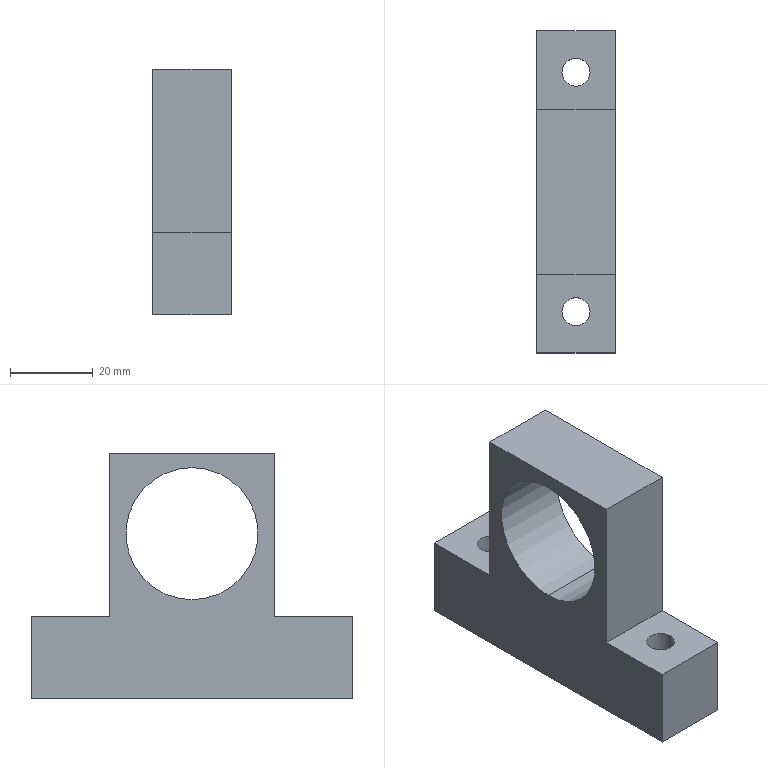Part | STEP file | PN_0052 secondary end seat | 1 solid | 16 faces | box 19 x 78 x 59.5 mm | volume 42927 mm3 | plane 10 | cylinder 6 | commonest cylinder face diameters 6.8 x4 32 x2
STEP:
#1=CARTESIAN_POINT('',(0.,0.,0.));
#2=DIRECTION('',(0.,0.,1.));
#3=DIRECTION('',(1.,0.,0.));
#4=AXIS2_PLACEMENT_3D('',#1,#2,#3);
#5=CARTESIAN_POINT('',(3.4,29.,0.));
#6=VERTEX_POINT('',#5);
#7=CARTESIAN_POINT('',(3.4,29.,20.));
#8=VERTEX_POINT('',#7);
#9=CARTESIAN_POINT('',(3.4,29.,20.));
#10=DIRECTION('',(0.,0.,1.));
#11=VECTOR('',#10,1.);
#12=LINE('',#9,#11);
#13=CARTESIAN_POINT('',(0.,29.,20.));
#14=DIRECTION('',(0.,0.,1.));
#15=DIRECTION('',(1.,0.,0.));
#16=AXIS2_PLACEMENT_3D('',#13,#14,#15);
#17=CYLINDRICAL_SURFACE('',#16,3.4);
#18=CARTESIAN_POINT('',(6.283,0.));
#19=DIRECTION('',(0.,1.));
#20=VECTOR('',#19,1.);
#21=LINE('',#18,#20);
#22=(GEOMETRIC_REPRESENTATION_CONTEXT(2)PARAMETRIC_REPRESENTATION_CONTEXT()REPRESENTATION_CONTEXT('',''));
#23=DEFINITIONAL_REPRESENTATION('',(#21),#22);
#24=PCURVE('',#17,#23);
#25=CARTESIAN_POINT('',(0.,29.,20.));
#26=DIRECTION('',(0.,0.,1.));
#27=DIRECTION('',(1.,0.,0.));
#28=AXIS2_PLACEMENT_3D('',#25,#26,#27);
#29=CYLINDRICAL_SURFACE('',#28,3.4);
#30=CARTESIAN_POINT('',(0.,0.));
#31=DIRECTION('',(0.,1.));
#32=VECTOR('',#31,1.);
#33=LINE('',#30,#32);
#34=(GEOMETRIC_REPRESENTATION_CONTEXT(2)PARAMETRIC_REPRESENTATION_CONTEXT()REPRESENTATION_CONTEXT('',''));
#35=DEFINITIONAL_REPRESENTATION('',(#33),#34);
#36=PCURVE('',#29,#35);
#37=SURFACE_CURVE('',#12,(#24,#36),.PCURVE_S1.);
#38=EDGE_CURVE('',#6,#8,#37,.T.);
#39=ORIENTED_EDGE('',*,*,#38,.T.);
#40=CARTESIAN_POINT('',(-3.4,29.,20.));
#41=VERTEX_POINT('',#40);
#42=CARTESIAN_POINT('',(0.,29.,20.));
#43=DIRECTION('',(0.,0.,1.));
#44=DIRECTION('',(1.,0.,0.));
#45=AXIS2_PLACEMENT_3D('',#42,#43,#44);
#46=CIRCLE('',#45,3.4);
#47=CARTESIAN_POINT('',(0.,0.));
#48=DIRECTION('',(1.,0.));
#49=VECTOR('',#48,1.);
#50=LINE('',#47,#49);
#51=(GEOMETRIC_REPRESENTATION_CONTEXT(2)PARAMETRIC_REPRESENTATION_CONTEXT()REPRESENTATION_CONTEXT('',''));
#52=DEFINITIONAL_REPRESENTATION('',(#50),#51);
#53=PCURVE('',#17,#52);
#54=CARTESIAN_POINT('',(9.5,39.,20.));
#55=DIRECTION('',(0.,0.,-1.));
#56=DIRECTION('',(0.,1.,0.));
#57=AXIS2_PLACEMENT_3D('',#54,#55,#56);
#58=PLANE('',#57);
#59=CARTESIAN_POINT('',(-10.,-6.1));
#60=CARTESIAN_POINT('',(-4.111,-6.1));
#61=CARTESIAN_POINT('',(-7.056,-11.2));
#62=CARTESIAN_POINT('',(-10.,-16.3));
#63=CARTESIAN_POINT('',(-12.944,-11.2));
#64=CARTESIAN_POINT('',(-15.889,-6.1));
#65=CARTESIAN_POINT('',(-10.,-6.1));
#66=(BOUNDED_CURVE()B_SPLINE_CURVE(2,(#59,#60,#61,#62,#63,#64,#65),.UNSPECIFIED.,.T.,.F.)B_SPLINE_CURVE_WITH_KNOTS((1,2,2,2,2,1),(-2.094,0.,2.094,4.189,6.283,8.378),.UNSPECIFIED.)CURVE()GEOMETRIC_REPRESENTATION_ITEM()RATIONAL_B_SPLINE_CURVE((1.,0.5,1.,0.5,1.,0.5,1.))REPRESENTATION_ITEM(''));
#67=(GEOMETRIC_REPRESENTATION_CONTEXT(2)PARAMETRIC_REPRESENTATION_CONTEXT()REPRESENTATION_CONTEXT('',''));
#68=DEFINITIONAL_REPRESENTATION('',(#66),#67);
#69=PCURVE('',#58,#68);
#70=SURFACE_CURVE('',#46,(#53,#69),.PCURVE_S1.);
#71=EDGE_CURVE('',#41,#8,#70,.T.);
#72=ORIENTED_EDGE('',*,*,#71,.F.);
#73=CARTESIAN_POINT('',(-3.4,29.,0.));
#74=VERTEX_POINT('',#73);
#75=CARTESIAN_POINT('',(-3.4,29.,20.));
#76=DIRECTION('',(0.,0.,1.));
#77=VECTOR('',#76,1.);
#78=LINE('',#75,#77);
#79=CARTESIAN_POINT('',(3.142,0.));
#80=DIRECTION('',(0.,1.));
#81=VECTOR('',#80,1.);
#82=LINE('',#79,#81);
#83=(GEOMETRIC_REPRESENTATION_CONTEXT(2)PARAMETRIC_REPRESENTATION_CONTEXT()REPRESENTATION_CONTEXT('',''));
#84=DEFINITIONAL_REPRESENTATION('',(#82),#83);
#85=PCURVE('',#17,#84);
#86=CARTESIAN_POINT('',(3.142,0.));
#87=DIRECTION('',(0.,1.));
#88=VECTOR('',#87,1.);
#89=LINE('',#86,#88);
#90=(GEOMETRIC_REPRESENTATION_CONTEXT(2)PARAMETRIC_REPRESENTATION_CONTEXT()REPRESENTATION_CONTEXT('',''));
#91=DEFINITIONAL_REPRESENTATION('',(#89),#90);
#92=PCURVE('',#29,#91);
#93=SURFACE_CURVE('',#78,(#85,#92),.PCURVE_S1.);
#94=EDGE_CURVE('',#74,#41,#93,.T.);
#95=ORIENTED_EDGE('',*,*,#94,.F.);
#96=CARTESIAN_POINT('',(0.,29.,0.));
#97=DIRECTION('',(0.,0.,1.));
#98=DIRECTION('',(1.,0.,0.));
#99=AXIS2_PLACEMENT_3D('',#96,#97,#98);
#100=CIRCLE('',#99,3.4);
#101=CARTESIAN_POINT('',(0.,-20.));
#102=DIRECTION('',(1.,0.));
#103=VECTOR('',#102,1.);
#104=LINE('',#101,#103);
#105=(GEOMETRIC_REPRESENTATION_CONTEXT(2)PARAMETRIC_REPRESENTATION_CONTEXT()REPRESENTATION_CONTEXT('',''));
#106=DEFINITIONAL_REPRESENTATION('',(#104),#105);
#107=PCURVE('',#17,#106);
#108=CARTESIAN_POINT('',(9.5,-39.,0.));
#109=DIRECTION('',(0.,0.,1.));
#110=DIRECTION('',(0.,-1.,0.));
#111=AXIS2_PLACEMENT_3D('',#108,#109,#110);
#112=PLANE('',#111);
#113=CARTESIAN_POINT('',(-68.,-9.5));
#114=DIRECTION('',(0.,1.));
#115=AXIS2_PLACEMENT_2D('',#113,#114);
#116=CIRCLE('',#115,3.4);
#117=(GEOMETRIC_REPRESENTATION_CONTEXT(2)PARAMETRIC_REPRESENTATION_CONTEXT()REPRESENTATION_CONTEXT('',''));
#118=DEFINITIONAL_REPRESENTATION('',(#116),#117);
#119=PCURVE('',#112,#118);
#120=SURFACE_CURVE('',#100,(#107,#119),.PCURVE_S1.);
#121=EDGE_CURVE('',#74,#6,#120,.T.);
#122=ORIENTED_EDGE('',*,*,#121,.T.);
#123=EDGE_LOOP('',(#39,#72,#95,#122));
#124=FACE_BOUND('',#123,.F.);
#125=ADVANCED_FACE('',(#124),#17,.F.);
#126=CARTESIAN_POINT('',(3.4,-29.,0.));
#127=VERTEX_POINT('',#126);
#128=CARTESIAN_POINT('',(3.4,-29.,20.));
#129=VERTEX_POINT('',#128);
#130=CARTESIAN_POINT('',(3.4,-29.,20.));
#131=DIRECTION('',(0.,0.,1.));
#132=VECTOR('',#131,1.);
#133=LINE('',#130,#132);
#134=CARTESIAN_POINT('',(0.,-29.,20.));
#135=DIRECTION('',(0.,0.,1.));
#136=DIRECTION('',(1.,0.,0.));
#137=AXIS2_PLACEMENT_3D('',#134,#135,#136);
#138=CYLINDRICAL_SURFACE('',#137,3.4);
#139=CARTESIAN_POINT('',(6.283,0.));
#140=DIRECTION('',(0.,1.));
#141=VECTOR('',#140,1.);
#142=LINE('',#139,#141);
#143=(GEOMETRIC_REPRESENTATION_CONTEXT(2)PARAMETRIC_REPRESENTATION_CONTEXT()REPRESENTATION_CONTEXT('',''));
#144=DEFINITIONAL_REPRESENTATION('',(#142),#143);
#145=PCURVE('',#138,#144);
#146=CARTESIAN_POINT('',(0.,-29.,20.));
#147=DIRECTION('',(0.,0.,1.));
#148=DIRECTION('',(1.,0.,0.));
#149=AXIS2_PLACEMENT_3D('',#146,#147,#148);
#150=CYLINDRICAL_SURFACE('',#149,3.4);
#151=CARTESIAN_POINT('',(0.,0.));
#152=DIRECTION('',(0.,1.));
#153=VECTOR('',#152,1.);
#154=LINE('',#151,#153);
#155=(GEOMETRIC_REPRESENTATION_CONTEXT(2)PARAMETRIC_REPRESENTATION_CONTEXT()REPRESENTATION_CONTEXT('',''));
#156=DEFINITIONAL_REPRESENTATION('',(#154),#155);
#157=PCURVE('',#150,#156);
#158=SURFACE_CURVE('',#133,(#145,#157),.PCURVE_S1.);
#159=EDGE_CURVE('',#127,#129,#158,.T.);
#160=ORIENTED_EDGE('',*,*,#159,.T.);
#161=CARTESIAN_POINT('',(-3.4,-29.,20.));
#162=VERTEX_POINT('',#161);
#163=CARTESIAN_POINT('',(0.,-29.,20.));
#164=DIRECTION('',(0.,0.,1.));
#165=DIRECTION('',(1.,0.,0.));
#166=AXIS2_PLACEMENT_3D('',#163,#164,#165);
#167=CIRCLE('',#166,3.4);
#168=CARTESIAN_POINT('',(0.,0.));
#169=DIRECTION('',(1.,0.));
#170=VECTOR('',#169,1.);
#171=LINE('',#168,#170);
#172=(GEOMETRIC_REPRESENTATION_CONTEXT(2)PARAMETRIC_REPRESENTATION_CONTEXT()REPRESENTATION_CONTEXT('',''));
#173=DEFINITIONAL_REPRESENTATION('',(#171),#172);
#174=PCURVE('',#138,#173);
#175=CARTESIAN_POINT('',(9.5,-20.,20.));
#176=DIRECTION('',(0.,0.,-1.));
#177=DIRECTION('',(0.,1.,0.));
#178=AXIS2_PLACEMENT_3D('',#175,#176,#177);
#179=PLANE('',#178);
#180=CARTESIAN_POINT('',(-9.,-6.1));
#181=CARTESIAN_POINT('',(-3.111,-6.1));
#182=CARTESIAN_POINT('',(-6.056,-11.2));
#183=CARTESIAN_POINT('',(-9.,-16.3));
#184=CARTESIAN_POINT('',(-11.944,-11.2));
#185=CARTESIAN_POINT('',(-14.889,-6.1));
#186=CARTESIAN_POINT('',(-9.,-6.1));
#187=(BOUNDED_CURVE()B_SPLINE_CURVE(2,(#180,#181,#182,#183,#184,#185,#186),.UNSPECIFIED.,.T.,.F.)B_SPLINE_CURVE_WITH_KNOTS((1,2,2,2,2,1),(-2.094,0.,2.094,4.189,6.283,8.378),.UNSPECIFIED.)CURVE()GEOMETRIC_REPRESENTATION_ITEM()RATIONAL_B_SPLINE_CURVE((1.,0.5,1.,0.5,1.,0.5,1.))REPRESENTATION_ITEM(''));
#188=(GEOMETRIC_REPRESENTATION_CONTEXT(2)PARAMETRIC_REPRESENTATION_CONTEXT()REPRESENTATION_CONTEXT('',''));
#189=DEFINITIONAL_REPRESENTATION('',(#187),#188);
#190=PCURVE('',#179,#189);
#191=SURFACE_CURVE('',#167,(#174,#190),.PCURVE_S1.);
#192=EDGE_CURVE('',#162,#129,#191,.T.);
#193=ORIENTED_EDGE('',*,*,#192,.F.);
#194=CARTESIAN_POINT('',(-3.4,-29.,0.));
#195=VERTEX_POINT('',#194);
#196=CARTESIAN_POINT('',(-3.4,-29.,20.));
#197=DIRECTION('',(0.,0.,1.));
#198=VECTOR('',#197,1.);
#199=LINE('',#196,#198);
#200=CARTESIAN_POINT('',(3.142,0.));
#201=DIRECTION('',(0.,1.));
#202=VECTOR('',#201,1.);
#203=LINE('',#200,#202);
#204=(GEOMETRIC_REPRESENTATION_CONTEXT(2)PARAMETRIC_REPRESENTATION_CONTEXT()REPRESENTATION_CONTEXT('',''));
#205=DEFINITIONAL_REPRESENTATION('',(#203),#204);
#206=PCURVE('',#138,#205);
#207=CARTESIAN_POINT('',(3.142,0.));
#208=DIRECTION('',(0.,1.));
#209=VECTOR('',#208,1.);
#210=LINE('',#207,#209);
#211=(GEOMETRIC_REPRESENTATION_CONTEXT(2)PARAMETRIC_REPRESENTATION_CONTEXT()REPRESENTATION_CONTEXT('',''));
#212=DEFINITIONAL_REPRESENTATION('',(#210),#211);
#213=PCURVE('',#150,#212);
#214=SURFACE_CURVE('',#199,(#206,#213),.PCURVE_S1.);
#215=EDGE_CURVE('',#195,#162,#214,.T.);
#216=ORIENTED_EDGE('',*,*,#215,.F.);
#217=CARTESIAN_POINT('',(0.,-29.,0.));
#218=DIRECTION('',(0.,0.,1.));
#219=DIRECTION('',(1.,0.,0.));
#220=AXIS2_PLACEMENT_3D('',#217,#218,#219);
#221=CIRCLE('',#220,3.4);
#222=CARTESIAN_POINT('',(0.,-20.));
#223=DIRECTION('',(1.,0.));
#224=VECTOR('',#223,1.);
#225=LINE('',#222,#224);
#226=(GEOMETRIC_REPRESENTATION_CONTEXT(2)PARAMETRIC_REPRESENTATION_CONTEXT()REPRESENTATION_CONTEXT('',''));
#227=DEFINITIONAL_REPRESENTATION('',(#225),#226);
#228=PCURVE('',#138,#227);
#229=CARTESIAN_POINT('',(-10.,-9.5));
#230=DIRECTION('',(0.,1.));
#231=AXIS2_PLACEMENT_2D('',#229,#230);
#232=CIRCLE('',#231,3.4);
#233=(GEOMETRIC_REPRESENTATION_CONTEXT(2)PARAMETRIC_REPRESENTATION_CONTEXT()REPRESENTATION_CONTEXT('',''));
#234=DEFINITIONAL_REPRESENTATION('',(#232),#233);
#235=PCURVE('',#112,#234);
#236=SURFACE_CURVE('',#221,(#228,#235),.PCURVE_S1.);
#237=EDGE_CURVE('',#195,#127,#236,.T.);
#238=ORIENTED_EDGE('',*,*,#237,.T.);
#239=EDGE_LOOP('',(#160,#193,#216,#238));
#240=FACE_BOUND('',#239,.F.);
#241=ADVANCED_FACE('',(#240),#138,.F.);
#242=CARTESIAN_POINT('',(-9.5,0.,24.));
#243=VERTEX_POINT('',#242);
#244=CARTESIAN_POINT('',(9.5,0.,24.));
#245=VERTEX_POINT('',#244);
#246=CARTESIAN_POINT('',(-9.5,0.,24.));
#247=DIRECTION('',(1.,0.,0.));
#248=VECTOR('',#247,1.);
#249=LINE('',#246,#248);
#250=CARTESIAN_POINT('',(-9.5,0.,40.));
#251=DIRECTION('',(1.,0.,0.));
#252=DIRECTION('',(0.,0.,-1.));
#253=AXIS2_PLACEMENT_3D('',#250,#251,#252);
#254=CYLINDRICAL_SURFACE('',#253,16.);
#255=CARTESIAN_POINT('',(6.283,0.));
#256=DIRECTION('',(0.,1.));
#257=VECTOR('',#256,1.);
#258=LINE('',#255,#257);
#259=(GEOMETRIC_REPRESENTATION_CONTEXT(2)PARAMETRIC_REPRESENTATION_CONTEXT()REPRESENTATION_CONTEXT('',''));
#260=DEFINITIONAL_REPRESENTATION('',(#258),#259);
#261=PCURVE('',#254,#260);
#262=CARTESIAN_POINT('',(-9.5,0.,40.));
#263=DIRECTION('',(1.,0.,0.));
#264=DIRECTION('',(0.,0.,-1.));
#265=AXIS2_PLACEMENT_3D('',#262,#263,#264);
#266=CYLINDRICAL_SURFACE('',#265,16.);
#267=CARTESIAN_POINT('',(0.,0.));
#268=DIRECTION('',(0.,1.));
#269=VECTOR('',#268,1.);
#270=LINE('',#267,#269);
#271=(GEOMETRIC_REPRESENTATION_CONTEXT(2)PARAMETRIC_REPRESENTATION_CONTEXT()REPRESENTATION_CONTEXT('',''));
#272=DEFINITIONAL_REPRESENTATION('',(#270),#271);
#273=PCURVE('',#266,#272);
#274=SURFACE_CURVE('',#249,(#261,#273),.PCURVE_S1.);
#275=EDGE_CURVE('',#243,#245,#274,.T.);
#276=ORIENTED_EDGE('',*,*,#275,.T.);
#277=CARTESIAN_POINT('',(9.5,0.,56.));
#278=VERTEX_POINT('',#277);
#279=CARTESIAN_POINT('',(9.5,0.,40.));
#280=DIRECTION('',(1.,0.,0.));
#281=DIRECTION('',(0.,0.,-1.));
#282=AXIS2_PLACEMENT_3D('',#279,#280,#281);
#283=CIRCLE('',#282,16.);
#284=CARTESIAN_POINT('',(0.,19.));
#285=DIRECTION('',(1.,0.));
#286=VECTOR('',#285,1.);
#287=LINE('',#284,#286);
#288=(GEOMETRIC_REPRESENTATION_CONTEXT(2)PARAMETRIC_REPRESENTATION_CONTEXT()REPRESENTATION_CONTEXT('',''));
#289=DEFINITIONAL_REPRESENTATION('',(#287),#288);
#290=PCURVE('',#254,#289);
#291=CARTESIAN_POINT('',(9.5,0.,0.));
#292=DIRECTION('',(1.,0.,0.));
#293=DIRECTION('',(0.,0.,-1.));
#294=AXIS2_PLACEMENT_3D('',#291,#292,#293);
#295=PLANE('',#294);
#296=CARTESIAN_POINT('',(-40.,0.));
#297=DIRECTION('',(1.,0.));
#298=AXIS2_PLACEMENT_2D('',#296,#297);
#299=CIRCLE('',#298,16.);
#300=(GEOMETRIC_REPRESENTATION_CONTEXT(2)PARAMETRIC_REPRESENTATION_CONTEXT()REPRESENTATION_CONTEXT('',''));
#301=DEFINITIONAL_REPRESENTATION('',(#299),#300);
#302=PCURVE('',#295,#301);
#303=SURFACE_CURVE('',#283,(#290,#302),.PCURVE_S1.);
#304=EDGE_CURVE('',#278,#245,#303,.T.);
#305=ORIENTED_EDGE('',*,*,#304,.F.);
#306=CARTESIAN_POINT('',(-9.5,0.,56.));
#307=VERTEX_POINT('',#306);
#308=CARTESIAN_POINT('',(-9.5,0.,56.));
#309=DIRECTION('',(1.,0.,0.));
#310=VECTOR('',#309,1.);
#311=LINE('',#308,#310);
#312=CARTESIAN_POINT('',(3.142,0.));
#313=DIRECTION('',(0.,1.));
#314=VECTOR('',#313,1.);
#315=LINE('',#312,#314);
#316=(GEOMETRIC_REPRESENTATION_CONTEXT(2)PARAMETRIC_REPRESENTATION_CONTEXT()REPRESENTATION_CONTEXT('',''));
#317=DEFINITIONAL_REPRESENTATION('',(#315),#316);
#318=PCURVE('',#254,#317);
#319=CARTESIAN_POINT('',(3.142,0.));
#320=DIRECTION('',(0.,1.));
#321=VECTOR('',#320,1.);
#322=LINE('',#319,#321);
#323=(GEOMETRIC_REPRESENTATION_CONTEXT(2)PARAMETRIC_REPRESENTATION_CONTEXT()REPRESENTATION_CONTEXT('',''));
#324=DEFINITIONAL_REPRESENTATION('',(#322),#323);
#325=PCURVE('',#266,#324);
#326=SURFACE_CURVE('',#311,(#318,#325),.PCURVE_S1.);
#327=EDGE_CURVE('',#307,#278,#326,.T.);
#328=ORIENTED_EDGE('',*,*,#327,.F.);
#329=CARTESIAN_POINT('',(-9.5,0.,40.));
#330=DIRECTION('',(1.,0.,0.));
#331=DIRECTION('',(0.,0.,-1.));
#332=AXIS2_PLACEMENT_3D('',#329,#330,#331);
#333=CIRCLE('',#332,16.);
#334=CARTESIAN_POINT('',(0.,0.));
#335=DIRECTION('',(1.,0.));
#336=VECTOR('',#335,1.);
#337=LINE('',#334,#336);
#338=(GEOMETRIC_REPRESENTATION_CONTEXT(2)PARAMETRIC_REPRESENTATION_CONTEXT()REPRESENTATION_CONTEXT('',''));
#339=DEFINITIONAL_REPRESENTATION('',(#337),#338);
#340=PCURVE('',#254,#339);
#341=CARTESIAN_POINT('',(-9.5,0.,0.));
#342=DIRECTION('',(1.,0.,0.));
#343=DIRECTION('',(0.,0.,-1.));
#344=AXIS2_PLACEMENT_3D('',#341,#342,#343);
#345=PLANE('',#344);
#346=CARTESIAN_POINT('',(-40.,0.));
#347=DIRECTION('',(1.,0.));
#348=AXIS2_PLACEMENT_2D('',#346,#347);
#349=CIRCLE('',#348,16.);
#350=(GEOMETRIC_REPRESENTATION_CONTEXT(2)PARAMETRIC_REPRESENTATION_CONTEXT()REPRESENTATION_CONTEXT('',''));
#351=DEFINITIONAL_REPRESENTATION('',(#349),#350);
#352=PCURVE('',#345,#351);
#353=SURFACE_CURVE('',#333,(#340,#352),.PCURVE_S1.);
#354=EDGE_CURVE('',#307,#243,#353,.T.);
#355=ORIENTED_EDGE('',*,*,#354,.T.);
#356=EDGE_LOOP('',(#276,#305,#328,#355));
#357=FACE_BOUND('',#356,.F.);
#358=ADVANCED_FACE('',(#357),#254,.F.);
#359=CARTESIAN_POINT('',(0.,29.,0.));
#360=DIRECTION('',(0.,0.,1.));
#361=DIRECTION('',(1.,0.,0.));
#362=AXIS2_PLACEMENT_3D('',#359,#360,#361);
#363=CIRCLE('',#362,3.4);
#364=CARTESIAN_POINT('',(-68.,-9.5));
#365=DIRECTION('',(0.,1.));
#366=AXIS2_PLACEMENT_2D('',#364,#365);
#367=CIRCLE('',#366,3.4);
#368=(GEOMETRIC_REPRESENTATION_CONTEXT(2)PARAMETRIC_REPRESENTATION_CONTEXT()REPRESENTATION_CONTEXT('',''));
#369=DEFINITIONAL_REPRESENTATION('',(#367),#368);
#370=PCURVE('',#112,#369);
#371=CARTESIAN_POINT('',(0.,-20.));
#372=DIRECTION('',(1.,0.));
#373=VECTOR('',#372,1.);
#374=LINE('',#371,#373);
#375=(GEOMETRIC_REPRESENTATION_CONTEXT(2)PARAMETRIC_REPRESENTATION_CONTEXT()REPRESENTATION_CONTEXT('',''));
#376=DEFINITIONAL_REPRESENTATION('',(#374),#375);
#377=PCURVE('',#29,#376);
#378=SURFACE_CURVE('',#363,(#370,#377),.PCURVE_S1.);
#379=EDGE_CURVE('',#6,#74,#378,.T.);
#380=ORIENTED_EDGE('',*,*,#379,.T.);
#381=ORIENTED_EDGE('',*,*,#121,.T.);
#382=EDGE_LOOP('',(#380,#381));
#383=FACE_BOUND('',#382,.T.);
#384=CARTESIAN_POINT('',(0.,-29.,0.));
#385=DIRECTION('',(0.,0.,1.));
#386=DIRECTION('',(1.,0.,0.));
#387=AXIS2_PLACEMENT_3D('',#384,#385,#386);
#388=CIRCLE('',#387,3.4);
#389=CARTESIAN_POINT('',(-10.,-9.5));
#390=DIRECTION('',(0.,1.));
#391=AXIS2_PLACEMENT_2D('',#389,#390);
#392=CIRCLE('',#391,3.4);
#393=(GEOMETRIC_REPRESENTATION_CONTEXT(2)PARAMETRIC_REPRESENTATION_CONTEXT()REPRESENTATION_CONTEXT('',''));
#394=DEFINITIONAL_REPRESENTATION('',(#392),#393);
#395=PCURVE('',#112,#394);
#396=CARTESIAN_POINT('',(0.,-20.));
#397=DIRECTION('',(1.,0.));
#398=VECTOR('',#397,1.);
#399=LINE('',#396,#398);
#400=(GEOMETRIC_REPRESENTATION_CONTEXT(2)PARAMETRIC_REPRESENTATION_CONTEXT()REPRESENTATION_CONTEXT('',''));
#401=DEFINITIONAL_REPRESENTATION('',(#399),#400);
#402=PCURVE('',#150,#401);
#403=SURFACE_CURVE('',#388,(#395,#402),.PCURVE_S1.);
#404=EDGE_CURVE('',#127,#195,#403,.T.);
#405=ORIENTED_EDGE('',*,*,#404,.T.);
#406=ORIENTED_EDGE('',*,*,#237,.T.);
#407=EDGE_LOOP('',(#405,#406));
#408=FACE_BOUND('',#407,.T.);
#409=CARTESIAN_POINT('',(-9.5,-39.,0.));
#410=VERTEX_POINT('',#409);
#411=CARTESIAN_POINT('',(-9.5,39.,0.));
#412=VERTEX_POINT('',#411);
#413=CARTESIAN_POINT('',(-9.5,-39.,0.));
#414=DIRECTION('',(0.,1.,0.));
#415=VECTOR('',#414,1.);
#416=LINE('',#413,#415);
#417=CARTESIAN_POINT('',(0.,-19.));
#418=DIRECTION('',(-1.,0.));
#419=VECTOR('',#418,1.);
#420=LINE('',#417,#419);
#421=(GEOMETRIC_REPRESENTATION_CONTEXT(2)PARAMETRIC_REPRESENTATION_CONTEXT()REPRESENTATION_CONTEXT('',''));
#422=DEFINITIONAL_REPRESENTATION('',(#420),#421);
#423=PCURVE('',#112,#422);
#424=CARTESIAN_POINT('',(0.,-39.));
#425=DIRECTION('',(0.,1.));
#426=VECTOR('',#425,1.);
#427=LINE('',#424,#426);
#428=(GEOMETRIC_REPRESENTATION_CONTEXT(2)PARAMETRIC_REPRESENTATION_CONTEXT()REPRESENTATION_CONTEXT('',''));
#429=DEFINITIONAL_REPRESENTATION('',(#427),#428);
#430=PCURVE('',#345,#429);
#431=SURFACE_CURVE('',#416,(#423,#430),.PCURVE_S1.);
#432=EDGE_CURVE('',#410,#412,#431,.T.);
#433=ORIENTED_EDGE('',*,*,#432,.T.);
#434=CARTESIAN_POINT('',(9.5,39.,0.));
#435=VERTEX_POINT('',#434);
#436=CARTESIAN_POINT('',(9.5,39.,0.));
#437=DIRECTION('',(-1.,0.,0.));
#438=VECTOR('',#437,1.);
#439=LINE('',#436,#438);
#440=CARTESIAN_POINT('',(-78.,0.));
#441=DIRECTION('',(0.,-1.));
#442=VECTOR('',#441,1.);
#443=LINE('',#440,#442);
#444=(GEOMETRIC_REPRESENTATION_CONTEXT(2)PARAMETRIC_REPRESENTATION_CONTEXT()REPRESENTATION_CONTEXT('',''));
#445=DEFINITIONAL_REPRESENTATION('',(#443),#444);
#446=PCURVE('',#112,#445);
#447=CARTESIAN_POINT('',(9.5,39.,0.));
#448=DIRECTION('',(0.,-1.,0.));
#449=DIRECTION('',(0.,0.,-1.));
#450=AXIS2_PLACEMENT_3D('',#447,#448,#449);
#451=PLANE('',#450);
#452=CARTESIAN_POINT('',(0.,0.));
#453=DIRECTION('',(0.,-1.));
#454=VECTOR('',#453,1.);
#455=LINE('',#452,#454);
#456=(GEOMETRIC_REPRESENTATION_CONTEXT(2)PARAMETRIC_REPRESENTATION_CONTEXT()REPRESENTATION_CONTEXT('',''));
#457=DEFINITIONAL_REPRESENTATION('',(#455),#456);
#458=PCURVE('',#451,#457);
#459=SURFACE_CURVE('',#439,(#446,#458),.PCURVE_S1.);
#460=EDGE_CURVE('',#435,#412,#459,.T.);
#461=ORIENTED_EDGE('',*,*,#460,.F.);
#462=CARTESIAN_POINT('',(9.5,-39.,0.));
#463=VERTEX_POINT('',#462);
#464=CARTESIAN_POINT('',(9.5,-39.,0.));
#465=DIRECTION('',(0.,1.,0.));
#466=VECTOR('',#465,1.);
#467=LINE('',#464,#466);
#468=CARTESIAN_POINT('',(0.,0.));
#469=DIRECTION('',(-1.,0.));
#470=VECTOR('',#469,1.);
#471=LINE('',#468,#470);
#472=(GEOMETRIC_REPRESENTATION_CONTEXT(2)PARAMETRIC_REPRESENTATION_CONTEXT()REPRESENTATION_CONTEXT('',''));
#473=DEFINITIONAL_REPRESENTATION('',(#471),#472);
#474=PCURVE('',#112,#473);
#475=CARTESIAN_POINT('',(0.,-39.));
#476=DIRECTION('',(0.,1.));
#477=VECTOR('',#476,1.);
#478=LINE('',#475,#477);
#479=(GEOMETRIC_REPRESENTATION_CONTEXT(2)PARAMETRIC_REPRESENTATION_CONTEXT()REPRESENTATION_CONTEXT('',''));
#480=DEFINITIONAL_REPRESENTATION('',(#478),#479);
#481=PCURVE('',#295,#480);
#482=SURFACE_CURVE('',#467,(#474,#481),.PCURVE_S1.);
#483=EDGE_CURVE('',#463,#435,#482,.T.);
#484=ORIENTED_EDGE('',*,*,#483,.F.);
#485=CARTESIAN_POINT('',(9.5,-39.,0.));
#486=DIRECTION('',(-1.,0.,0.));
#487=VECTOR('',#486,1.);
#488=LINE('',#485,#487);
#489=CARTESIAN_POINT('',(0.,0.));
#490=DIRECTION('',(0.,-1.));
#491=VECTOR('',#490,1.);
#492=LINE('',#489,#491);
#493=(GEOMETRIC_REPRESENTATION_CONTEXT(2)PARAMETRIC_REPRESENTATION_CONTEXT()REPRESENTATION_CONTEXT('',''));
#494=DEFINITIONAL_REPRESENTATION('',(#492),#493);
#495=PCURVE('',#112,#494);
#496=CARTESIAN_POINT('',(9.5,-39.,0.));
#497=DIRECTION('',(0.,1.,0.));
#498=DIRECTION('',(0.,0.,1.));
#499=AXIS2_PLACEMENT_3D('',#496,#497,#498);
#500=PLANE('',#499);
#501=CARTESIAN_POINT('',(0.,0.));
#502=DIRECTION('',(0.,-1.));
#503=VECTOR('',#502,1.);
#504=LINE('',#501,#503);
#505=(GEOMETRIC_REPRESENTATION_CONTEXT(2)PARAMETRIC_REPRESENTATION_CONTEXT()REPRESENTATION_CONTEXT('',''));
#506=DEFINITIONAL_REPRESENTATION('',(#504),#505);
#507=PCURVE('',#500,#506);
#508=SURFACE_CURVE('',#488,(#495,#507),.PCURVE_S1.);
#509=EDGE_CURVE('',#463,#410,#508,.T.);
#510=ORIENTED_EDGE('',*,*,#509,.T.);
#511=EDGE_LOOP('',(#433,#461,#484,#510));
#512=FACE_BOUND('',#511,.T.);
#513=ADVANCED_FACE('',(#383,#408,#512),#112,.F.);
#514=CARTESIAN_POINT('',(-9.5,39.,20.));
#515=VERTEX_POINT('',#514);
#516=CARTESIAN_POINT('',(-9.5,39.,0.));
#517=DIRECTION('',(0.,0.,1.));
#518=VECTOR('',#517,1.);
#519=LINE('',#516,#518);
#520=CARTESIAN_POINT('',(0.,-19.));
#521=DIRECTION('',(-1.,0.));
#522=VECTOR('',#521,1.);
#523=LINE('',#520,#522);
#524=(GEOMETRIC_REPRESENTATION_CONTEXT(2)PARAMETRIC_REPRESENTATION_CONTEXT()REPRESENTATION_CONTEXT('',''));
#525=DEFINITIONAL_REPRESENTATION('',(#523),#524);
#526=PCURVE('',#451,#525);
#527=CARTESIAN_POINT('',(0.,39.));
#528=DIRECTION('',(-1.,0.));
#529=VECTOR('',#528,1.);
#530=LINE('',#527,#529);
#531=(GEOMETRIC_REPRESENTATION_CONTEXT(2)PARAMETRIC_REPRESENTATION_CONTEXT()REPRESENTATION_CONTEXT('',''));
#532=DEFINITIONAL_REPRESENTATION('',(#530),#531);
#533=PCURVE('',#345,#532);
#534=SURFACE_CURVE('',#519,(#526,#533),.PCURVE_S1.);
#535=EDGE_CURVE('',#412,#515,#534,.T.);
#536=ORIENTED_EDGE('',*,*,#535,.T.);
#537=CARTESIAN_POINT('',(9.5,39.,20.));
#538=VERTEX_POINT('',#537);
#539=CARTESIAN_POINT('',(9.5,39.,20.));
#540=DIRECTION('',(-1.,0.,0.));
#541=VECTOR('',#540,1.);
#542=LINE('',#539,#541);
#543=CARTESIAN_POINT('',(-20.,0.));
#544=DIRECTION('',(0.,-1.));
#545=VECTOR('',#544,1.);
#546=LINE('',#543,#545);
#547=(GEOMETRIC_REPRESENTATION_CONTEXT(2)PARAMETRIC_REPRESENTATION_CONTEXT()REPRESENTATION_CONTEXT('',''));
#548=DEFINITIONAL_REPRESENTATION('',(#546),#547);
#549=PCURVE('',#451,#548);
#550=CARTESIAN_POINT('',(0.,0.));
#551=DIRECTION('',(0.,-1.));
#552=VECTOR('',#551,1.);
#553=LINE('',#550,#552);
#554=(GEOMETRIC_REPRESENTATION_CONTEXT(2)PARAMETRIC_REPRESENTATION_CONTEXT()REPRESENTATION_CONTEXT('',''));
#555=DEFINITIONAL_REPRESENTATION('',(#553),#554);
#556=PCURVE('',#58,#555);
#557=SURFACE_CURVE('',#542,(#549,#556),.PCURVE_S1.);
#558=EDGE_CURVE('',#538,#515,#557,.T.);
#559=ORIENTED_EDGE('',*,*,#558,.F.);
#560=CARTESIAN_POINT('',(9.5,39.,0.));
#561=DIRECTION('',(0.,0.,1.));
#562=VECTOR('',#561,1.);
#563=LINE('',#560,#562);
#564=CARTESIAN_POINT('',(0.,0.));
#565=DIRECTION('',(-1.,0.));
#566=VECTOR('',#565,1.);
#567=LINE('',#564,#566);
#568=(GEOMETRIC_REPRESENTATION_CONTEXT(2)PARAMETRIC_REPRESENTATION_CONTEXT()REPRESENTATION_CONTEXT('',''));
#569=DEFINITIONAL_REPRESENTATION('',(#567),#568);
#570=PCURVE('',#451,#569);
#571=CARTESIAN_POINT('',(0.,39.));
#572=DIRECTION('',(-1.,0.));
#573=VECTOR('',#572,1.);
#574=LINE('',#571,#573);
#575=(GEOMETRIC_REPRESENTATION_CONTEXT(2)PARAMETRIC_REPRESENTATION_CONTEXT()REPRESENTATION_CONTEXT('',''));
#576=DEFINITIONAL_REPRESENTATION('',(#574),#575);
#577=PCURVE('',#295,#576);
#578=SURFACE_CURVE('',#563,(#570,#577),.PCURVE_S1.);
#579=EDGE_CURVE('',#435,#538,#578,.T.);
#580=ORIENTED_EDGE('',*,*,#579,.F.);
#581=ORIENTED_EDGE('',*,*,#460,.T.);
#582=EDGE_LOOP('',(#536,#559,#580,#581));
#583=FACE_BOUND('',#582,.T.);
#584=ADVANCED_FACE('',(#583),#451,.F.);
#585=CARTESIAN_POINT('',(0.,29.,20.));
#586=DIRECTION('',(0.,0.,1.));
#587=DIRECTION('',(1.,0.,0.));
#588=AXIS2_PLACEMENT_3D('',#585,#586,#587);
#589=CIRCLE('',#588,3.4);
#590=CARTESIAN_POINT('',(-10.,-6.1));
#591=CARTESIAN_POINT('',(-4.111,-6.1));
#592=CARTESIAN_POINT('',(-7.056,-11.2));
#593=CARTESIAN_POINT('',(-10.,-16.3));
#594=CARTESIAN_POINT('',(-12.944,-11.2));
#595=CARTESIAN_POINT('',(-15.889,-6.1));
#596=CARTESIAN_POINT('',(-10.,-6.1));
#597=(BOUNDED_CURVE()B_SPLINE_CURVE(2,(#590,#591,#592,#593,#594,#595,#596),.UNSPECIFIED.,.T.,.F.)B_SPLINE_CURVE_WITH_KNOTS((1,2,2,2,2,1),(-2.094,0.,2.094,4.189,6.283,8.378),.UNSPECIFIED.)CURVE()GEOMETRIC_REPRESENTATION_ITEM()RATIONAL_B_SPLINE_CURVE((1.,0.5,1.,0.5,1.,0.5,1.))REPRESENTATION_ITEM(''));
#598=(GEOMETRIC_REPRESENTATION_CONTEXT(2)PARAMETRIC_REPRESENTATION_CONTEXT()REPRESENTATION_CONTEXT('',''));
#599=DEFINITIONAL_REPRESENTATION('',(#597),#598);
#600=PCURVE('',#58,#599);
#601=CARTESIAN_POINT('',(0.,0.));
#602=DIRECTION('',(1.,0.));
#603=VECTOR('',#602,1.);
#604=LINE('',#601,#603);
#605=(GEOMETRIC_REPRESENTATION_CONTEXT(2)PARAMETRIC_REPRESENTATION_CONTEXT()REPRESENTATION_CONTEXT('',''));
#606=DEFINITIONAL_REPRESENTATION('',(#604),#605);
#607=PCURVE('',#29,#606);
#608=SURFACE_CURVE('',#589,(#600,#607),.PCURVE_S1.);
#609=EDGE_CURVE('',#8,#41,#608,.T.);
#610=ORIENTED_EDGE('',*,*,#609,.F.);
#611=ORIENTED_EDGE('',*,*,#71,.F.);
#612=EDGE_LOOP('',(#610,#611));
#613=FACE_BOUND('',#612,.T.);
#614=CARTESIAN_POINT('',(-9.5,20.,20.));
#615=VERTEX_POINT('',#614);
#616=CARTESIAN_POINT('',(-9.5,39.,20.));
#617=DIRECTION('',(0.,-1.,0.));
#618=VECTOR('',#617,1.);
#619=LINE('',#616,#618);
#620=CARTESIAN_POINT('',(0.,-19.));
#621=DIRECTION('',(-1.,0.));
#622=VECTOR('',#621,1.);
#623=LINE('',#620,#622);
#624=(GEOMETRIC_REPRESENTATION_CONTEXT(2)PARAMETRIC_REPRESENTATION_CONTEXT()REPRESENTATION_CONTEXT('',''));
#625=DEFINITIONAL_REPRESENTATION('',(#623),#624);
#626=PCURVE('',#58,#625);
#627=CARTESIAN_POINT('',(-20.,39.));
#628=DIRECTION('',(0.,-1.));
#629=VECTOR('',#628,1.);
#630=LINE('',#627,#629);
#631=(GEOMETRIC_REPRESENTATION_CONTEXT(2)PARAMETRIC_REPRESENTATION_CONTEXT()REPRESENTATION_CONTEXT('',''));
#632=DEFINITIONAL_REPRESENTATION('',(#630),#631);
#633=PCURVE('',#345,#632);
#634=SURFACE_CURVE('',#619,(#626,#633),.PCURVE_S1.);
#635=EDGE_CURVE('',#515,#615,#634,.T.);
#636=ORIENTED_EDGE('',*,*,#635,.T.);
#637=CARTESIAN_POINT('',(9.5,20.,20.));
#638=VERTEX_POINT('',#637);
#639=CARTESIAN_POINT('',(9.5,20.,20.));
#640=DIRECTION('',(-1.,0.,0.));
#641=VECTOR('',#640,1.);
#642=LINE('',#639,#641);
#643=CARTESIAN_POINT('',(-19.,0.));
#644=DIRECTION('',(0.,-1.));
#645=VECTOR('',#644,1.);
#646=LINE('',#643,#645);
#647=(GEOMETRIC_REPRESENTATION_CONTEXT(2)PARAMETRIC_REPRESENTATION_CONTEXT()REPRESENTATION_CONTEXT('',''));
#648=DEFINITIONAL_REPRESENTATION('',(#646),#647);
#649=PCURVE('',#58,#648);
#650=CARTESIAN_POINT('',(9.5,20.,20.));
#651=DIRECTION('',(0.,-1.,0.));
#652=DIRECTION('',(0.,0.,-1.));
#653=AXIS2_PLACEMENT_3D('',#650,#651,#652);
#654=PLANE('',#653);
#655=CARTESIAN_POINT('',(0.,0.));
#656=DIRECTION('',(0.,-1.));
#657=VECTOR('',#656,1.);
#658=LINE('',#655,#657);
#659=(GEOMETRIC_REPRESENTATION_CONTEXT(2)PARAMETRIC_REPRESENTATION_CONTEXT()REPRESENTATION_CONTEXT('',''));
#660=DEFINITIONAL_REPRESENTATION('',(#658),#659);
#661=PCURVE('',#654,#660);
#662=SURFACE_CURVE('',#642,(#649,#661),.PCURVE_S1.);
#663=EDGE_CURVE('',#638,#615,#662,.T.);
#664=ORIENTED_EDGE('',*,*,#663,.F.);
#665=CARTESIAN_POINT('',(9.5,39.,20.));
#666=DIRECTION('',(0.,-1.,0.));
#667=VECTOR('',#666,1.);
#668=LINE('',#665,#667);
#669=CARTESIAN_POINT('',(0.,0.));
#670=DIRECTION('',(-1.,0.));
#671=VECTOR('',#670,1.);
#672=LINE('',#669,#671);
#673=(GEOMETRIC_REPRESENTATION_CONTEXT(2)PARAMETRIC_REPRESENTATION_CONTEXT()REPRESENTATION_CONTEXT('',''));
#674=DEFINITIONAL_REPRESENTATION('',(#672),#673);
#675=PCURVE('',#58,#674);
#676=CARTESIAN_POINT('',(-20.,39.));
#677=DIRECTION('',(0.,-1.));
#678=VECTOR('',#677,1.);
#679=LINE('',#676,#678);
#680=(GEOMETRIC_REPRESENTATION_CONTEXT(2)PARAMETRIC_REPRESENTATION_CONTEXT()REPRESENTATION_CONTEXT('',''));
#681=DEFINITIONAL_REPRESENTATION('',(#679),#680);
#682=PCURVE('',#295,#681);
#683=SURFACE_CURVE('',#668,(#675,#682),.PCURVE_S1.);
#684=EDGE_CURVE('',#538,#638,#683,.T.);
#685=ORIENTED_EDGE('',*,*,#684,.F.);
#686=ORIENTED_EDGE('',*,*,#558,.T.);
#687=EDGE_LOOP('',(#636,#664,#685,#686));
#688=FACE_BOUND('',#687,.T.);
#689=ADVANCED_FACE('',(#613,#688),#58,.F.);
#690=CARTESIAN_POINT('',(-9.5,20.,59.5));
#691=VERTEX_POINT('',#690);
#692=CARTESIAN_POINT('',(-9.5,20.,20.));
#693=DIRECTION('',(0.,0.,1.));
#694=VECTOR('',#693,1.);
#695=LINE('',#692,#694);
#696=CARTESIAN_POINT('',(0.,-19.));
#697=DIRECTION('',(-1.,0.));
#698=VECTOR('',#697,1.);
#699=LINE('',#696,#698);
#700=(GEOMETRIC_REPRESENTATION_CONTEXT(2)PARAMETRIC_REPRESENTATION_CONTEXT()REPRESENTATION_CONTEXT('',''));
#701=DEFINITIONAL_REPRESENTATION('',(#699),#700);
#702=PCURVE('',#654,#701);
#703=CARTESIAN_POINT('',(-20.,20.));
#704=DIRECTION('',(-1.,0.));
#705=VECTOR('',#704,1.);
#706=LINE('',#703,#705);
#707=(GEOMETRIC_REPRESENTATION_CONTEXT(2)PARAMETRIC_REPRESENTATION_CONTEXT()REPRESENTATION_CONTEXT('',''));
#708=DEFINITIONAL_REPRESENTATION('',(#706),#707);
#709=PCURVE('',#345,#708);
#710=SURFACE_CURVE('',#695,(#702,#709),.PCURVE_S1.);
#711=EDGE_CURVE('',#615,#691,#710,.T.);
#712=ORIENTED_EDGE('',*,*,#711,.T.);
#713=CARTESIAN_POINT('',(9.5,20.,59.5));
#714=VERTEX_POINT('',#713);
#715=CARTESIAN_POINT('',(9.5,20.,59.5));
#716=DIRECTION('',(-1.,0.,0.));
#717=VECTOR('',#716,1.);
#718=LINE('',#715,#717);
#719=CARTESIAN_POINT('',(-39.5,0.));
#720=DIRECTION('',(0.,-1.));
#721=VECTOR('',#720,1.);
#722=LINE('',#719,#721);
#723=(GEOMETRIC_REPRESENTATION_CONTEXT(2)PARAMETRIC_REPRESENTATION_CONTEXT()REPRESENTATION_CONTEXT('',''));
#724=DEFINITIONAL_REPRESENTATION('',(#722),#723);
#725=PCURVE('',#654,#724);
#726=CARTESIAN_POINT('',(9.5,20.,59.5));
#727=DIRECTION('',(0.,0.,-1.));
#728=DIRECTION('',(0.,1.,0.));
#729=AXIS2_PLACEMENT_3D('',#726,#727,#728);
#730=PLANE('',#729);
#731=CARTESIAN_POINT('',(0.,0.));
#732=DIRECTION('',(0.,-1.));
#733=VECTOR('',#732,1.);
#734=LINE('',#731,#733);
#735=(GEOMETRIC_REPRESENTATION_CONTEXT(2)PARAMETRIC_REPRESENTATION_CONTEXT()REPRESENTATION_CONTEXT('',''));
#736=DEFINITIONAL_REPRESENTATION('',(#734),#735);
#737=PCURVE('',#730,#736);
#738=SURFACE_CURVE('',#718,(#725,#737),.PCURVE_S1.);
#739=EDGE_CURVE('',#714,#691,#738,.T.);
#740=ORIENTED_EDGE('',*,*,#739,.F.);
#741=CARTESIAN_POINT('',(9.5,20.,20.));
#742=DIRECTION('',(0.,0.,1.));
#743=VECTOR('',#742,1.);
#744=LINE('',#741,#743);
#745=CARTESIAN_POINT('',(0.,0.));
#746=DIRECTION('',(-1.,0.));
#747=VECTOR('',#746,1.);
#748=LINE('',#745,#747);
#749=(GEOMETRIC_REPRESENTATION_CONTEXT(2)PARAMETRIC_REPRESENTATION_CONTEXT()REPRESENTATION_CONTEXT('',''));
#750=DEFINITIONAL_REPRESENTATION('',(#748),#749);
#751=PCURVE('',#654,#750);
#752=CARTESIAN_POINT('',(-20.,20.));
#753=DIRECTION('',(-1.,0.));
#754=VECTOR('',#753,1.);
#755=LINE('',#752,#754);
#756=(GEOMETRIC_REPRESENTATION_CONTEXT(2)PARAMETRIC_REPRESENTATION_CONTEXT()REPRESENTATION_CONTEXT('',''));
#757=DEFINITIONAL_REPRESENTATION('',(#755),#756);
#758=PCURVE('',#295,#757);
#759=SURFACE_CURVE('',#744,(#751,#758),.PCURVE_S1.);
#760=EDGE_CURVE('',#638,#714,#759,.T.);
#761=ORIENTED_EDGE('',*,*,#760,.F.);
#762=ORIENTED_EDGE('',*,*,#663,.T.);
#763=EDGE_LOOP('',(#712,#740,#761,#762));
#764=FACE_BOUND('',#763,.T.);
#765=ADVANCED_FACE('',(#764),#654,.F.);
#766=CARTESIAN_POINT('',(-9.5,-20.,59.5));
#767=VERTEX_POINT('',#766);
#768=CARTESIAN_POINT('',(-9.5,20.,59.5));
#769=DIRECTION('',(0.,-1.,0.));
#770=VECTOR('',#769,1.);
#771=LINE('',#768,#770);
#772=CARTESIAN_POINT('',(0.,-19.));
#773=DIRECTION('',(-1.,0.));
#774=VECTOR('',#773,1.);
#775=LINE('',#772,#774);
#776=(GEOMETRIC_REPRESENTATION_CONTEXT(2)PARAMETRIC_REPRESENTATION_CONTEXT()REPRESENTATION_CONTEXT('',''));
#777=DEFINITIONAL_REPRESENTATION('',(#775),#776);
#778=PCURVE('',#730,#777);
#779=CARTESIAN_POINT('',(-59.5,20.));
#780=DIRECTION('',(0.,-1.));
#781=VECTOR('',#780,1.);
#782=LINE('',#779,#781);
#783=(GEOMETRIC_REPRESENTATION_CONTEXT(2)PARAMETRIC_REPRESENTATION_CONTEXT()REPRESENTATION_CONTEXT('',''));
#784=DEFINITIONAL_REPRESENTATION('',(#782),#783);
#785=PCURVE('',#345,#784);
#786=SURFACE_CURVE('',#771,(#778,#785),.PCURVE_S1.);
#787=EDGE_CURVE('',#691,#767,#786,.T.);
#788=ORIENTED_EDGE('',*,*,#787,.T.);
#789=CARTESIAN_POINT('',(9.5,-20.,59.5));
#790=VERTEX_POINT('',#789);
#791=CARTESIAN_POINT('',(9.5,-20.,59.5));
#792=DIRECTION('',(-1.,0.,0.));
#793=VECTOR('',#792,1.);
#794=LINE('',#791,#793);
#795=CARTESIAN_POINT('',(-40.,0.));
#796=DIRECTION('',(0.,-1.));
#797=VECTOR('',#796,1.);
#798=LINE('',#795,#797);
#799=(GEOMETRIC_REPRESENTATION_CONTEXT(2)PARAMETRIC_REPRESENTATION_CONTEXT()REPRESENTATION_CONTEXT('',''));
#800=DEFINITIONAL_REPRESENTATION('',(#798),#799);
#801=PCURVE('',#730,#800);
#802=CARTESIAN_POINT('',(9.5,-20.,59.5));
#803=DIRECTION('',(0.,1.,0.));
#804=DIRECTION('',(0.,0.,1.));
#805=AXIS2_PLACEMENT_3D('',#802,#803,#804);
#806=PLANE('',#805);
#807=CARTESIAN_POINT('',(0.,0.));
#808=DIRECTION('',(0.,-1.));
#809=VECTOR('',#808,1.);
#810=LINE('',#807,#809);
#811=(GEOMETRIC_REPRESENTATION_CONTEXT(2)PARAMETRIC_REPRESENTATION_CONTEXT()REPRESENTATION_CONTEXT('',''));
#812=DEFINITIONAL_REPRESENTATION('',(#810),#811);
#813=PCURVE('',#806,#812);
#814=SURFACE_CURVE('',#794,(#801,#813),.PCURVE_S1.);
#815=EDGE_CURVE('',#790,#767,#814,.T.);
#816=ORIENTED_EDGE('',*,*,#815,.F.);
#817=CARTESIAN_POINT('',(9.5,20.,59.5));
#818=DIRECTION('',(0.,-1.,0.));
#819=VECTOR('',#818,1.);
#820=LINE('',#817,#819);
#821=CARTESIAN_POINT('',(0.,0.));
#822=DIRECTION('',(-1.,0.));
#823=VECTOR('',#822,1.);
#824=LINE('',#821,#823);
#825=(GEOMETRIC_REPRESENTATION_CONTEXT(2)PARAMETRIC_REPRESENTATION_CONTEXT()REPRESENTATION_CONTEXT('',''));
#826=DEFINITIONAL_REPRESENTATION('',(#824),#825);
#827=PCURVE('',#730,#826);
#828=CARTESIAN_POINT('',(-59.5,20.));
#829=DIRECTION('',(0.,-1.));
#830=VECTOR('',#829,1.);
#831=LINE('',#828,#830);
#832=(GEOMETRIC_REPRESENTATION_CONTEXT(2)PARAMETRIC_REPRESENTATION_CONTEXT()REPRESENTATION_CONTEXT('',''));
#833=DEFINITIONAL_REPRESENTATION('',(#831),#832);
#834=PCURVE('',#295,#833);
#835=SURFACE_CURVE('',#820,(#827,#834),.PCURVE_S1.);
#836=EDGE_CURVE('',#714,#790,#835,.T.);
#837=ORIENTED_EDGE('',*,*,#836,.F.);
#838=ORIENTED_EDGE('',*,*,#739,.T.);
#839=EDGE_LOOP('',(#788,#816,#837,#838));
#840=FACE_BOUND('',#839,.T.);
#841=ADVANCED_FACE('',(#840),#730,.F.);
#842=CARTESIAN_POINT('',(-9.5,-20.,20.));
#843=VERTEX_POINT('',#842);
#844=CARTESIAN_POINT('',(-9.5,-20.,59.5));
#845=DIRECTION('',(0.,0.,-1.));
#846=VECTOR('',#845,1.);
#847=LINE('',#844,#846);
#848=CARTESIAN_POINT('',(0.,-19.));
#849=DIRECTION('',(-1.,0.));
#850=VECTOR('',#849,1.);
#851=LINE('',#848,#850);
#852=(GEOMETRIC_REPRESENTATION_CONTEXT(2)PARAMETRIC_REPRESENTATION_CONTEXT()REPRESENTATION_CONTEXT('',''));
#853=DEFINITIONAL_REPRESENTATION('',(#851),#852);
#854=PCURVE('',#806,#853);
#855=CARTESIAN_POINT('',(-59.5,-20.));
#856=DIRECTION('',(1.,0.));
#857=VECTOR('',#856,1.);
#858=LINE('',#855,#857);
#859=(GEOMETRIC_REPRESENTATION_CONTEXT(2)PARAMETRIC_REPRESENTATION_CONTEXT()REPRESENTATION_CONTEXT('',''));
#860=DEFINITIONAL_REPRESENTATION('',(#858),#859);
#861=PCURVE('',#345,#860);
#862=SURFACE_CURVE('',#847,(#854,#861),.PCURVE_S1.);
#863=EDGE_CURVE('',#767,#843,#862,.T.);
#864=ORIENTED_EDGE('',*,*,#863,.T.);
#865=CARTESIAN_POINT('',(9.5,-20.,20.));
#866=VERTEX_POINT('',#865);
#867=CARTESIAN_POINT('',(9.5,-20.,20.));
#868=DIRECTION('',(-1.,0.,0.));
#869=VECTOR('',#868,1.);
#870=LINE('',#867,#869);
#871=CARTESIAN_POINT('',(-39.5,0.));
#872=DIRECTION('',(0.,-1.));
#873=VECTOR('',#872,1.);
#874=LINE('',#871,#873);
#875=(GEOMETRIC_REPRESENTATION_CONTEXT(2)PARAMETRIC_REPRESENTATION_CONTEXT()REPRESENTATION_CONTEXT('',''));
#876=DEFINITIONAL_REPRESENTATION('',(#874),#875);
#877=PCURVE('',#806,#876);
#878=CARTESIAN_POINT('',(0.,0.));
#879=DIRECTION('',(0.,-1.));
#880=VECTOR('',#879,1.);
#881=LINE('',#878,#880);
#882=(GEOMETRIC_REPRESENTATION_CONTEXT(2)PARAMETRIC_REPRESENTATION_CONTEXT()REPRESENTATION_CONTEXT('',''));
#883=DEFINITIONAL_REPRESENTATION('',(#881),#882);
#884=PCURVE('',#179,#883);
#885=SURFACE_CURVE('',#870,(#877,#884),.PCURVE_S1.);
#886=EDGE_CURVE('',#866,#843,#885,.T.);
#887=ORIENTED_EDGE('',*,*,#886,.F.);
#888=CARTESIAN_POINT('',(9.5,-20.,59.5));
#889=DIRECTION('',(0.,0.,-1.));
#890=VECTOR('',#889,1.);
#891=LINE('',#888,#890);
#892=CARTESIAN_POINT('',(0.,0.));
#893=DIRECTION('',(-1.,0.));
#894=VECTOR('',#893,1.);
#895=LINE('',#892,#894);
#896=(GEOMETRIC_REPRESENTATION_CONTEXT(2)PARAMETRIC_REPRESENTATION_CONTEXT()REPRESENTATION_CONTEXT('',''));
#897=DEFINITIONAL_REPRESENTATION('',(#895),#896);
#898=PCURVE('',#806,#897);
#899=CARTESIAN_POINT('',(-59.5,-20.));
#900=DIRECTION('',(1.,0.));
#901=VECTOR('',#900,1.);
#902=LINE('',#899,#901);
#903=(GEOMETRIC_REPRESENTATION_CONTEXT(2)PARAMETRIC_REPRESENTATION_CONTEXT()REPRESENTATION_CONTEXT('',''));
#904=DEFINITIONAL_REPRESENTATION('',(#902),#903);
#905=PCURVE('',#295,#904);
#906=SURFACE_CURVE('',#891,(#898,#905),.PCURVE_S1.);
#907=EDGE_CURVE('',#790,#866,#906,.T.);
#908=ORIENTED_EDGE('',*,*,#907,.F.);
#909=ORIENTED_EDGE('',*,*,#815,.T.);
#910=EDGE_LOOP('',(#864,#887,#908,#909));
#911=FACE_BOUND('',#910,.T.);
#912=ADVANCED_FACE('',(#911),#806,.F.);
#913=CARTESIAN_POINT('',(0.,-29.,20.));
#914=DIRECTION('',(0.,0.,1.));
#915=DIRECTION('',(1.,0.,0.));
#916=AXIS2_PLACEMENT_3D('',#913,#914,#915);
#917=CIRCLE('',#916,3.4);
#918=CARTESIAN_POINT('',(-9.,-6.1));
#919=CARTESIAN_POINT('',(-3.111,-6.1));
#920=CARTESIAN_POINT('',(-6.056,-11.2));
#921=CARTESIAN_POINT('',(-9.,-16.3));
#922=CARTESIAN_POINT('',(-11.944,-11.2));
#923=CARTESIAN_POINT('',(-14.889,-6.1));
#924=CARTESIAN_POINT('',(-9.,-6.1));
#925=(BOUNDED_CURVE()B_SPLINE_CURVE(2,(#918,#919,#920,#921,#922,#923,#924),.UNSPECIFIED.,.T.,.F.)B_SPLINE_CURVE_WITH_KNOTS((1,2,2,2,2,1),(-2.094,0.,2.094,4.189,6.283,8.378),.UNSPECIFIED.)CURVE()GEOMETRIC_REPRESENTATION_ITEM()RATIONAL_B_SPLINE_CURVE((1.,0.5,1.,0.5,1.,0.5,1.))REPRESENTATION_ITEM(''));
#926=(GEOMETRIC_REPRESENTATION_CONTEXT(2)PARAMETRIC_REPRESENTATION_CONTEXT()REPRESENTATION_CONTEXT('',''));
#927=DEFINITIONAL_REPRESENTATION('',(#925),#926);
#928=PCURVE('',#179,#927);
#929=CARTESIAN_POINT('',(0.,0.));
#930=DIRECTION('',(1.,0.));
#931=VECTOR('',#930,1.);
#932=LINE('',#929,#931);
#933=(GEOMETRIC_REPRESENTATION_CONTEXT(2)PARAMETRIC_REPRESENTATION_CONTEXT()REPRESENTATION_CONTEXT('',''));
#934=DEFINITIONAL_REPRESENTATION('',(#932),#933);
#935=PCURVE('',#150,#934);
#936=SURFACE_CURVE('',#917,(#928,#935),.PCURVE_S1.);
#937=EDGE_CURVE('',#129,#162,#936,.T.);
#938=ORIENTED_EDGE('',*,*,#937,.F.);
#939=ORIENTED_EDGE('',*,*,#192,.F.);
#940=EDGE_LOOP('',(#938,#939));
#941=FACE_BOUND('',#940,.T.);
#942=CARTESIAN_POINT('',(-9.5,-39.,20.));
#943=VERTEX_POINT('',#942);
#944=CARTESIAN_POINT('',(-9.5,-20.,20.));
#945=DIRECTION('',(0.,-1.,0.));
#946=VECTOR('',#945,1.);
#947=LINE('',#944,#946);
#948=CARTESIAN_POINT('',(0.,-19.));
#949=DIRECTION('',(-1.,0.));
#950=VECTOR('',#949,1.);
#951=LINE('',#948,#950);
#952=(GEOMETRIC_REPRESENTATION_CONTEXT(2)PARAMETRIC_REPRESENTATION_CONTEXT()REPRESENTATION_CONTEXT('',''));
#953=DEFINITIONAL_REPRESENTATION('',(#951),#952);
#954=PCURVE('',#179,#953);
#955=CARTESIAN_POINT('',(-20.,-20.));
#956=DIRECTION('',(0.,-1.));
#957=VECTOR('',#956,1.);
#958=LINE('',#955,#957);
#959=(GEOMETRIC_REPRESENTATION_CONTEXT(2)PARAMETRIC_REPRESENTATION_CONTEXT()REPRESENTATION_CONTEXT('',''));
#960=DEFINITIONAL_REPRESENTATION('',(#958),#959);
#961=PCURVE('',#345,#960);
#962=SURFACE_CURVE('',#947,(#954,#961),.PCURVE_S1.);
#963=EDGE_CURVE('',#843,#943,#962,.T.);
#964=ORIENTED_EDGE('',*,*,#963,.T.);
#965=CARTESIAN_POINT('',(9.5,-39.,20.));
#966=VERTEX_POINT('',#965);
#967=CARTESIAN_POINT('',(9.5,-39.,20.));
#968=DIRECTION('',(-1.,0.,0.));
#969=VECTOR('',#968,1.);
#970=LINE('',#967,#969);
#971=CARTESIAN_POINT('',(-19.,0.));
#972=DIRECTION('',(0.,-1.));
#973=VECTOR('',#972,1.);
#974=LINE('',#971,#973);
#975=(GEOMETRIC_REPRESENTATION_CONTEXT(2)PARAMETRIC_REPRESENTATION_CONTEXT()REPRESENTATION_CONTEXT('',''));
#976=DEFINITIONAL_REPRESENTATION('',(#974),#975);
#977=PCURVE('',#179,#976);
#978=CARTESIAN_POINT('',(20.,0.));
#979=DIRECTION('',(0.,-1.));
#980=VECTOR('',#979,1.);
#981=LINE('',#978,#980);
#982=(GEOMETRIC_REPRESENTATION_CONTEXT(2)PARAMETRIC_REPRESENTATION_CONTEXT()REPRESENTATION_CONTEXT('',''));
#983=DEFINITIONAL_REPRESENTATION('',(#981),#982);
#984=PCURVE('',#500,#983);
#985=SURFACE_CURVE('',#970,(#977,#984),.PCURVE_S1.);
#986=EDGE_CURVE('',#966,#943,#985,.T.);
#987=ORIENTED_EDGE('',*,*,#986,.F.);
#988=CARTESIAN_POINT('',(9.5,-20.,20.));
#989=DIRECTION('',(0.,-1.,0.));
#990=VECTOR('',#989,1.);
#991=LINE('',#988,#990);
#992=CARTESIAN_POINT('',(0.,0.));
#993=DIRECTION('',(-1.,0.));
#994=VECTOR('',#993,1.);
#995=LINE('',#992,#994);
#996=(GEOMETRIC_REPRESENTATION_CONTEXT(2)PARAMETRIC_REPRESENTATION_CONTEXT()REPRESENTATION_CONTEXT('',''));
#997=DEFINITIONAL_REPRESENTATION('',(#995),#996);
#998=PCURVE('',#179,#997);
#999=CARTESIAN_POINT('',(-20.,-20.));
#1000=DIRECTION('',(0.,-1.));
#1001=VECTOR('',#1000,1.);
#1002=LINE('',#999,#1001);
#1003=(GEOMETRIC_REPRESENTATION_CONTEXT(2)PARAMETRIC_REPRESENTATION_CONTEXT()REPRESENTATION_CONTEXT('',''));
#1004=DEFINITIONAL_REPRESENTATION('',(#1002),#1003);
#1005=PCURVE('',#295,#1004);
#1006=SURFACE_CURVE('',#991,(#998,#1005),.PCURVE_S1.);
#1007=EDGE_CURVE('',#866,#966,#1006,.T.);
#1008=ORIENTED_EDGE('',*,*,#1007,.F.);
#1009=ORIENTED_EDGE('',*,*,#886,.T.);
#1010=EDGE_LOOP('',(#964,#987,#1008,#1009));
#1011=FACE_BOUND('',#1010,.T.);
#1012=ADVANCED_FACE('',(#941,#1011),#179,.F.);
#1013=CARTESIAN_POINT('',(-9.5,-39.,0.));
#1014=DIRECTION('',(0.,0.,-1.));
#1015=VECTOR('',#1014,1.);
#1016=LINE('',#1013,#1015);
#1017=CARTESIAN_POINT('',(0.,-19.));
#1018=DIRECTION('',(-1.,0.));
#1019=VECTOR('',#1018,1.);
#1020=LINE('',#1017,#1019);
#1021=(GEOMETRIC_REPRESENTATION_CONTEXT(2)PARAMETRIC_REPRESENTATION_CONTEXT()REPRESENTATION_CONTEXT('',''));
#1022=DEFINITIONAL_REPRESENTATION('',(#1020),#1021);
#1023=PCURVE('',#500,#1022);
#1024=CARTESIAN_POINT('',(0.,-39.));
#1025=DIRECTION('',(1.,0.));
#1026=VECTOR('',#1025,1.);
#1027=LINE('',#1024,#1026);
#1028=(GEOMETRIC_REPRESENTATION_CONTEXT(2)PARAMETRIC_REPRESENTATION_CONTEXT()REPRESENTATION_CONTEXT('',''));
#1029=DEFINITIONAL_REPRESENTATION('',(#1027),#1028);
#1030=PCURVE('',#345,#1029);
#1031=SURFACE_CURVE('',#1016,(#1023,#1030),.PCURVE_S1.);
#1032=EDGE_CURVE('',#943,#410,#1031,.T.);
#1033=ORIENTED_EDGE('',*,*,#1032,.T.);
#1034=ORIENTED_EDGE('',*,*,#509,.F.);
#1035=CARTESIAN_POINT('',(9.5,-39.,0.));
#1036=DIRECTION('',(0.,0.,-1.));
#1037=VECTOR('',#1036,1.);
#1038=LINE('',#1035,#1037);
#1039=CARTESIAN_POINT('',(0.,0.));
#1040=DIRECTION('',(-1.,0.));
#1041=VECTOR('',#1040,1.);
#1042=LINE('',#1039,#1041);
#1043=(GEOMETRIC_REPRESENTATION_CONTEXT(2)PARAMETRIC_REPRESENTATION_CONTEXT()REPRESENTATION_CONTEXT('',''));
#1044=DEFINITIONAL_REPRESENTATION('',(#1042),#1043);
#1045=PCURVE('',#500,#1044);
#1046=CARTESIAN_POINT('',(0.,-39.));
#1047=DIRECTION('',(1.,0.));
#1048=VECTOR('',#1047,1.);
#1049=LINE('',#1046,#1048);
#1050=(GEOMETRIC_REPRESENTATION_CONTEXT(2)PARAMETRIC_REPRESENTATION_CONTEXT()REPRESENTATION_CONTEXT('',''));
#1051=DEFINITIONAL_REPRESENTATION('',(#1049),#1050);
#1052=PCURVE('',#295,#1051);
#1053=SURFACE_CURVE('',#1038,(#1045,#1052),.PCURVE_S1.);
#1054=EDGE_CURVE('',#966,#463,#1053,.T.);
#1055=ORIENTED_EDGE('',*,*,#1054,.F.);
#1056=ORIENTED_EDGE('',*,*,#986,.T.);
#1057=EDGE_LOOP('',(#1033,#1034,#1055,#1056));
#1058=FACE_BOUND('',#1057,.T.);
#1059=ADVANCED_FACE('',(#1058),#500,.F.);
#1060=CARTESIAN_POINT('',(9.5,0.,40.));
#1061=DIRECTION('',(1.,0.,0.));
#1062=DIRECTION('',(0.,0.,-1.));
#1063=AXIS2_PLACEMENT_3D('',#1060,#1061,#1062);
#1064=CIRCLE('',#1063,16.);
#1065=CARTESIAN_POINT('',(-40.,0.));
#1066=DIRECTION('',(1.,0.));
#1067=AXIS2_PLACEMENT_2D('',#1065,#1066);
#1068=CIRCLE('',#1067,16.);
#1069=(GEOMETRIC_REPRESENTATION_CONTEXT(2)PARAMETRIC_REPRESENTATION_CONTEXT()REPRESENTATION_CONTEXT('',''));
#1070=DEFINITIONAL_REPRESENTATION('',(#1068),#1069);
#1071=PCURVE('',#295,#1070);
#1072=CARTESIAN_POINT('',(0.,19.));
#1073=DIRECTION('',(1.,0.));
#1074=VECTOR('',#1073,1.);
#1075=LINE('',#1072,#1074);
#1076=(GEOMETRIC_REPRESENTATION_CONTEXT(2)PARAMETRIC_REPRESENTATION_CONTEXT()REPRESENTATION_CONTEXT('',''));
#1077=DEFINITIONAL_REPRESENTATION('',(#1075),#1076);
#1078=PCURVE('',#266,#1077);
#1079=SURFACE_CURVE('',#1064,(#1071,#1078),.PCURVE_S1.);
#1080=EDGE_CURVE('',#245,#278,#1079,.T.);
#1081=ORIENTED_EDGE('',*,*,#1080,.F.);
#1082=ORIENTED_EDGE('',*,*,#304,.F.);
#1083=EDGE_LOOP('',(#1081,#1082));
#1084=FACE_BOUND('',#1083,.T.);
#1085=ORIENTED_EDGE('',*,*,#483,.T.);
#1086=ORIENTED_EDGE('',*,*,#579,.T.);
#1087=ORIENTED_EDGE('',*,*,#684,.T.);
#1088=ORIENTED_EDGE('',*,*,#760,.T.);
#1089=ORIENTED_EDGE('',*,*,#836,.T.);
#1090=ORIENTED_EDGE('',*,*,#907,.T.);
#1091=ORIENTED_EDGE('',*,*,#1007,.T.);
#1092=ORIENTED_EDGE('',*,*,#1054,.T.);
#1093=EDGE_LOOP('',(#1085,#1086,#1087,#1088,#1089,#1090,#1091,#1092));
#1094=FACE_BOUND('',#1093,.T.);
#1095=ADVANCED_FACE('',(#1084,#1094),#295,.T.);
#1096=CARTESIAN_POINT('',(-9.5,0.,40.));
#1097=DIRECTION('',(1.,0.,0.));
#1098=DIRECTION('',(0.,0.,-1.));
#1099=AXIS2_PLACEMENT_3D('',#1096,#1097,#1098);
#1100=CIRCLE('',#1099,16.);
#1101=CARTESIAN_POINT('',(-40.,0.));
#1102=DIRECTION('',(1.,0.));
#1103=AXIS2_PLACEMENT_2D('',#1101,#1102);
#1104=CIRCLE('',#1103,16.);
#1105=(GEOMETRIC_REPRESENTATION_CONTEXT(2)PARAMETRIC_REPRESENTATION_CONTEXT()REPRESENTATION_CONTEXT('',''));
#1106=DEFINITIONAL_REPRESENTATION('',(#1104),#1105);
#1107=PCURVE('',#345,#1106);
#1108=CARTESIAN_POINT('',(0.,0.));
#1109=DIRECTION('',(1.,0.));
#1110=VECTOR('',#1109,1.);
#1111=LINE('',#1108,#1110);
#1112=(GEOMETRIC_REPRESENTATION_CONTEXT(2)PARAMETRIC_REPRESENTATION_CONTEXT()REPRESENTATION_CONTEXT('',''));
#1113=DEFINITIONAL_REPRESENTATION('',(#1111),#1112);
#1114=PCURVE('',#266,#1113);
#1115=SURFACE_CURVE('',#1100,(#1107,#1114),.PCURVE_S1.);
#1116=EDGE_CURVE('',#243,#307,#1115,.T.);
#1117=ORIENTED_EDGE('',*,*,#1116,.T.);
#1118=ORIENTED_EDGE('',*,*,#354,.T.);
#1119=EDGE_LOOP('',(#1117,#1118));
#1120=FACE_BOUND('',#1119,.T.);
#1121=ORIENTED_EDGE('',*,*,#432,.F.);
#1122=ORIENTED_EDGE('',*,*,#1032,.F.);
#1123=ORIENTED_EDGE('',*,*,#963,.F.);
#1124=ORIENTED_EDGE('',*,*,#863,.F.);
#1125=ORIENTED_EDGE('',*,*,#787,.F.);
#1126=ORIENTED_EDGE('',*,*,#711,.F.);
#1127=ORIENTED_EDGE('',*,*,#635,.F.);
#1128=ORIENTED_EDGE('',*,*,#535,.F.);
#1129=EDGE_LOOP('',(#1121,#1122,#1123,#1124,#1125,#1126,#1127,#1128));
#1130=FACE_BOUND('',#1129,.T.);
#1131=ADVANCED_FACE('',(#1120,#1130),#345,.F.);
#1132=ORIENTED_EDGE('',*,*,#1080,.F.);
#1133=ORIENTED_EDGE('',*,*,#275,.F.);
#1134=ORIENTED_EDGE('',*,*,#1116,.T.);
#1135=ORIENTED_EDGE('',*,*,#327,.T.);
#1136=EDGE_LOOP('',(#1132,#1133,#1134,#1135));
#1137=FACE_BOUND('',#1136,.F.);
#1138=ADVANCED_FACE('',(#1137),#266,.F.);
#1139=ORIENTED_EDGE('',*,*,#937,.F.);
#1140=ORIENTED_EDGE('',*,*,#159,.F.);
#1141=ORIENTED_EDGE('',*,*,#404,.T.);
#1142=ORIENTED_EDGE('',*,*,#215,.T.);
#1143=EDGE_LOOP('',(#1139,#1140,#1141,#1142));
#1144=FACE_BOUND('',#1143,.F.);
#1145=ADVANCED_FACE('',(#1144),#150,.F.);
#1146=ORIENTED_EDGE('',*,*,#609,.F.);
#1147=ORIENTED_EDGE('',*,*,#38,.F.);
#1148=ORIENTED_EDGE('',*,*,#379,.T.);
#1149=ORIENTED_EDGE('',*,*,#94,.T.);
#1150=EDGE_LOOP('',(#1146,#1147,#1148,#1149));
#1151=FACE_BOUND('',#1150,.F.);
#1152=ADVANCED_FACE('',(#1151),#29,.F.);
#1153=CLOSED_SHELL('',(#125,#241,#358,#513,#584,#689,#765,#841,#912,#1012,#1059,#1095,#1131,#1138,#1145,#1152));
#1154=MANIFOLD_SOLID_BREP('',#1153);
#1155=(LENGTH_UNIT()NAMED_UNIT(*)SI_UNIT(.MILLI.,.METRE.));
#1156=UNCERTAINTY_MEASURE_WITH_UNIT(LENGTH_MEASURE(0.0000001),#1155,'','');
#1157=(NAMED_UNIT(*)PLANE_ANGLE_UNIT()SI_UNIT($,.RADIAN.));
#1158=(NAMED_UNIT(*)SI_UNIT($,.STERADIAN.)SOLID_ANGLE_UNIT());
#1159=(GEOMETRIC_REPRESENTATION_CONTEXT(3)GLOBAL_UNCERTAINTY_ASSIGNED_CONTEXT((#1156))GLOBAL_UNIT_ASSIGNED_CONTEXT((#1155,#1157,#1158))REPRESENTATION_CONTEXT('',''));
#1160=ADVANCED_BREP_SHAPE_REPRESENTATION('',(#4,#1154),#1159);